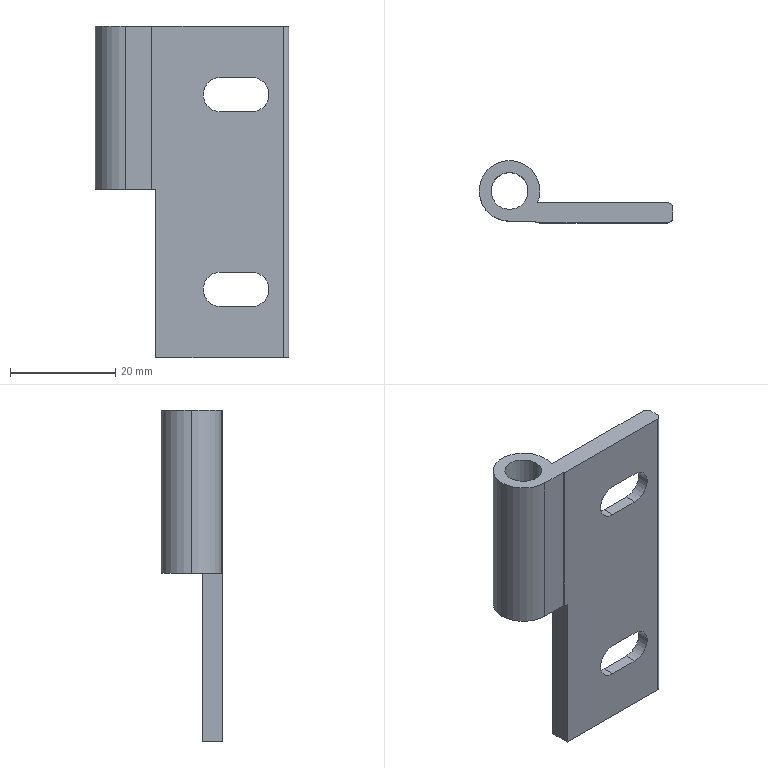Part | NX | features BREP 1 | 1 solid | 38 faces | box 36.75 x 11.75 x 63 mm | volume 7446 mm3 | cylinder 19 | plane 19 | commonest cylinder face diameters 6.5 x6 11 x6 11.5 x3 2 x2 7 x2
STEP:
#1=CARTESIAN_POINT('',(12.5,-3.7,18.5));
#2=VERTEX_POINT('',#1);
#3=CARTESIAN_POINT('',(18.,-3.7,24.));
#4=VERTEX_POINT('',#3);
#5=CARTESIAN_POINT('',(18.,-3.7,18.5));
#6=DIRECTION('',(0.,1.,0.));
#7=DIRECTION('',(-1.,0.,0.));
#8=AXIS2_PLACEMENT_3D('',#5,#6,#7);
#9=CIRCLE('',#8,5.5);
#10=EDGE_CURVE('',#2,#4,#9,.T.);
#11=ORIENTED_EDGE('',*,*,#10,.F.);
#12=CARTESIAN_POINT('',(12.5,-2.2,18.5));
#13=VERTEX_POINT('',#12);
#14=CARTESIAN_POINT('',(12.5,-3.7,18.5));
#15=DIRECTION('',(0.,1.,0.));
#16=VECTOR('',#15,1000.);
#17=LINE('',#14,#16);
#18=EDGE_CURVE('',#2,#13,#17,.T.);
#19=ORIENTED_EDGE('',*,*,#18,.T.);
#20=CARTESIAN_POINT('',(18.,-2.2,24.));
#21=VERTEX_POINT('',#20);
#22=CARTESIAN_POINT('',(18.,-2.2,18.5));
#23=DIRECTION('',(0.,1.,0.));
#24=DIRECTION('',(-1.,0.,0.));
#25=AXIS2_PLACEMENT_3D('',#22,#23,#24);
#26=CIRCLE('',#25,5.5);
#27=EDGE_CURVE('',#13,#21,#26,.T.);
#28=ORIENTED_EDGE('',*,*,#27,.T.);
#29=CARTESIAN_POINT('',(18.,-3.7,24.));
#30=DIRECTION('',(0.,1.,0.));
#31=VECTOR('',#30,1000.);
#32=LINE('',#29,#31);
#33=EDGE_CURVE('',#4,#21,#32,.T.);
#34=ORIENTED_EDGE('',*,*,#33,.F.);
#35=EDGE_LOOP('',(#11,#19,#28,#34));
#36=FACE_BOUND('',#35,.T.);
#37=CARTESIAN_POINT('',(18.,-3.7,18.5));
#38=DIRECTION('',(0.,1.,0.));
#39=DIRECTION('',(-1.,0.,0.));
#40=AXIS2_PLACEMENT_3D('',#37,#38,#39);
#41=CYLINDRICAL_SURFACE('',#40,5.5);
#42=ADVANCED_FACE('',(#36),#41,.F.);
#43=CARTESIAN_POINT('',(12.5,-3.7,-18.5));
#44=VERTEX_POINT('',#43);
#45=CARTESIAN_POINT('',(18.,-3.7,-13.));
#46=VERTEX_POINT('',#45);
#47=CARTESIAN_POINT('',(18.,-3.7,-18.5));
#48=DIRECTION('',(0.,1.,0.));
#49=DIRECTION('',(-1.,0.,0.));
#50=AXIS2_PLACEMENT_3D('',#47,#48,#49);
#51=CIRCLE('',#50,5.5);
#52=EDGE_CURVE('',#44,#46,#51,.T.);
#53=ORIENTED_EDGE('',*,*,#52,.F.);
#54=CARTESIAN_POINT('',(12.5,-2.2,-18.5));
#55=VERTEX_POINT('',#54);
#56=CARTESIAN_POINT('',(12.5,-3.7,-18.5));
#57=DIRECTION('',(0.,1.,0.));
#58=VECTOR('',#57,1000.);
#59=LINE('',#56,#58);
#60=EDGE_CURVE('',#44,#55,#59,.T.);
#61=ORIENTED_EDGE('',*,*,#60,.T.);
#62=CARTESIAN_POINT('',(18.,-2.2,-13.));
#63=VERTEX_POINT('',#62);
#64=CARTESIAN_POINT('',(18.,-2.2,-18.5));
#65=DIRECTION('',(0.,1.,0.));
#66=DIRECTION('',(-1.,0.,0.));
#67=AXIS2_PLACEMENT_3D('',#64,#65,#66);
#68=CIRCLE('',#67,5.5);
#69=EDGE_CURVE('',#55,#63,#68,.T.);
#70=ORIENTED_EDGE('',*,*,#69,.T.);
#71=CARTESIAN_POINT('',(18.,-3.7,-13.));
#72=DIRECTION('',(0.,1.,0.));
#73=VECTOR('',#72,1000.);
#74=LINE('',#71,#73);
#75=EDGE_CURVE('',#46,#63,#74,.T.);
#76=ORIENTED_EDGE('',*,*,#75,.F.);
#77=EDGE_LOOP('',(#53,#61,#70,#76));
#78=FACE_BOUND('',#77,.T.);
#79=CARTESIAN_POINT('',(18.,-3.7,-18.5));
#80=DIRECTION('',(0.,1.,0.));
#81=DIRECTION('',(-1.,0.,0.));
#82=AXIS2_PLACEMENT_3D('',#79,#80,#81);
#83=CYLINDRICAL_SURFACE('',#82,5.5);
#84=ADVANCED_FACE('',(#78),#83,.F.);
#85=CARTESIAN_POINT('',(-3.5,0.,31.5));
#86=VERTEX_POINT('',#85);
#87=CARTESIAN_POINT('',(3.5,0.,31.5));
#88=VERTEX_POINT('',#87);
#89=CARTESIAN_POINT('',(0.,0.,31.5));
#90=DIRECTION('',(0.,0.,1.));
#91=DIRECTION('',(1.,0.,0.));
#92=AXIS2_PLACEMENT_3D('',#89,#90,#91);
#93=CIRCLE('',#92,3.5);
#94=EDGE_CURVE('',#86,#88,#93,.T.);
#95=ORIENTED_EDGE('',*,*,#94,.T.);
#96=CARTESIAN_POINT('',(3.5,0.,0.5));
#97=VERTEX_POINT('',#96);
#98=CARTESIAN_POINT('',(3.5,0.,31.5));
#99=DIRECTION('',(0.,0.,-1.));
#100=VECTOR('',#99,1000.);
#101=LINE('',#98,#100);
#102=EDGE_CURVE('',#88,#97,#101,.T.);
#103=ORIENTED_EDGE('',*,*,#102,.T.);
#104=CARTESIAN_POINT('',(-3.5,0.,0.5));
#105=VERTEX_POINT('',#104);
#106=CARTESIAN_POINT('',(0.,0.,0.5));
#107=DIRECTION('',(0.,0.,1.));
#108=DIRECTION('',(1.,0.,0.));
#109=AXIS2_PLACEMENT_3D('',#106,#107,#108);
#110=CIRCLE('',#109,3.5);
#111=EDGE_CURVE('',#105,#97,#110,.T.);
#112=ORIENTED_EDGE('',*,*,#111,.F.);
#113=CARTESIAN_POINT('',(-3.5,0.,31.5));
#114=DIRECTION('',(0.,0.,-1.));
#115=VECTOR('',#114,1000.);
#116=LINE('',#113,#115);
#117=EDGE_CURVE('',#86,#105,#116,.T.);
#118=ORIENTED_EDGE('',*,*,#117,.F.);
#119=EDGE_LOOP('',(#95,#103,#112,#118));
#120=FACE_BOUND('',#119,.T.);
#121=CARTESIAN_POINT('',(0.,0.,31.5));
#122=DIRECTION('',(0.,0.,-1.));
#123=DIRECTION('',(-1.,0.,0.));
#124=AXIS2_PLACEMENT_3D('',#121,#122,#123);
#125=CYLINDRICAL_SURFACE('',#124,3.5);
#126=ADVANCED_FACE('',(#120),#125,.F.);
#127=CARTESIAN_POINT('',(5.75,0.,31.5));
#128=VERTEX_POINT('',#127);
#129=CARTESIAN_POINT('',(-5.75,0.,31.5));
#130=VERTEX_POINT('',#129);
#131=CARTESIAN_POINT('',(0.,0.,31.5));
#132=DIRECTION('',(0.,0.,1.));
#133=DIRECTION('',(1.,0.,0.));
#134=AXIS2_PLACEMENT_3D('',#131,#132,#133);
#135=CIRCLE('',#134,5.75);
#136=EDGE_CURVE('',#128,#130,#135,.T.);
#137=ORIENTED_EDGE('',*,*,#136,.F.);
#138=CARTESIAN_POINT('',(5.75,0.,0.5));
#139=VERTEX_POINT('',#138);
#140=CARTESIAN_POINT('',(5.75,0.,31.5));
#141=DIRECTION('',(0.,0.,-1.));
#142=VECTOR('',#141,1000.);
#143=LINE('',#140,#142);
#144=EDGE_CURVE('',#128,#139,#143,.T.);
#145=ORIENTED_EDGE('',*,*,#144,.T.);
#146=CARTESIAN_POINT('',(-5.75,0.,0.5));
#147=VERTEX_POINT('',#146);
#148=CARTESIAN_POINT('',(0.,0.,0.5));
#149=DIRECTION('',(0.,0.,1.));
#150=DIRECTION('',(1.,0.,0.));
#151=AXIS2_PLACEMENT_3D('',#148,#149,#150);
#152=CIRCLE('',#151,5.75);
#153=EDGE_CURVE('',#139,#147,#152,.T.);
#154=ORIENTED_EDGE('',*,*,#153,.T.);
#155=CARTESIAN_POINT('',(-5.75,0.,31.5));
#156=DIRECTION('',(0.,0.,-1.));
#157=VECTOR('',#156,1000.);
#158=LINE('',#155,#157);
#159=EDGE_CURVE('',#130,#147,#158,.T.);
#160=ORIENTED_EDGE('',*,*,#159,.F.);
#161=EDGE_LOOP('',(#137,#145,#154,#160));
#162=FACE_BOUND('',#161,.T.);
#163=CARTESIAN_POINT('',(0.,0.,31.5));
#164=DIRECTION('',(0.,0.,-1.));
#165=DIRECTION('',(-1.,0.,0.));
#166=AXIS2_PLACEMENT_3D('',#163,#164,#165);
#167=CYLINDRICAL_SURFACE('',#166,5.75);
#168=ADVANCED_FACE('',(#162),#167,.T.);
#169=CARTESIAN_POINT('',(0.,-5.75,31.5));
#170=VERTEX_POINT('',#169);
#171=CARTESIAN_POINT('',(0.,0.,31.5));
#172=DIRECTION('',(0.,0.,1.));
#173=DIRECTION('',(1.,0.,0.));
#174=AXIS2_PLACEMENT_3D('',#171,#172,#173);
#175=CIRCLE('',#174,5.75);
#176=EDGE_CURVE('',#130,#170,#175,.T.);
#177=ORIENTED_EDGE('',*,*,#176,.F.);
#178=ORIENTED_EDGE('',*,*,#159,.T.);
#179=CARTESIAN_POINT('',(0.,-5.75,0.5));
#180=VERTEX_POINT('',#179);
#181=CARTESIAN_POINT('',(0.,0.,0.5));
#182=DIRECTION('',(0.,0.,1.));
#183=DIRECTION('',(1.,0.,0.));
#184=AXIS2_PLACEMENT_3D('',#181,#182,#183);
#185=CIRCLE('',#184,5.75);
#186=EDGE_CURVE('',#147,#180,#185,.T.);
#187=ORIENTED_EDGE('',*,*,#186,.T.);
#188=CARTESIAN_POINT('',(0.,-5.75,31.5));
#189=DIRECTION('',(0.,0.,-1.));
#190=VECTOR('',#189,1000.);
#191=LINE('',#188,#190);
#192=EDGE_CURVE('',#170,#180,#191,.T.);
#193=ORIENTED_EDGE('',*,*,#192,.F.);
#194=EDGE_LOOP('',(#177,#178,#187,#193));
#195=FACE_BOUND('',#194,.T.);
#196=CARTESIAN_POINT('',(0.,0.,31.5));
#197=DIRECTION('',(0.,0.,-1.));
#198=DIRECTION('',(-1.,0.,0.));
#199=AXIS2_PLACEMENT_3D('',#196,#197,#198);
#200=CYLINDRICAL_SURFACE('',#199,5.75);
#201=ADVANCED_FACE('',(#195),#200,.T.);
#202=CARTESIAN_POINT('',(14.75,-6.,-18.5));
#203=VERTEX_POINT('',#202);
#204=CARTESIAN_POINT('',(18.,-6.,-15.25));
#205=VERTEX_POINT('',#204);
#206=CARTESIAN_POINT('',(18.,-6.,-18.5));
#207=DIRECTION('',(0.,1.,0.));
#208=DIRECTION('',(-1.,0.,0.));
#209=AXIS2_PLACEMENT_3D('',#206,#207,#208);
#210=CIRCLE('',#209,3.25);
#211=EDGE_CURVE('',#203,#205,#210,.T.);
#212=ORIENTED_EDGE('',*,*,#211,.F.);
#213=CARTESIAN_POINT('',(14.75,-3.7,-18.5));
#214=VERTEX_POINT('',#213);
#215=CARTESIAN_POINT('',(14.75,-6.,-18.5));
#216=DIRECTION('',(0.,1.,0.));
#217=VECTOR('',#216,1000.);
#218=LINE('',#215,#217);
#219=EDGE_CURVE('',#203,#214,#218,.T.);
#220=ORIENTED_EDGE('',*,*,#219,.T.);
#221=CARTESIAN_POINT('',(18.,-3.7,-15.25));
#222=VERTEX_POINT('',#221);
#223=CARTESIAN_POINT('',(18.,-3.7,-18.5));
#224=DIRECTION('',(0.,-1.,0.));
#225=DIRECTION('',(-1.,0.,0.));
#226=AXIS2_PLACEMENT_3D('',#223,#224,#225);
#227=CIRCLE('',#226,3.25);
#228=EDGE_CURVE('',#222,#214,#227,.T.);
#229=ORIENTED_EDGE('',*,*,#228,.F.);
#230=CARTESIAN_POINT('',(18.,-6.,-15.25));
#231=DIRECTION('',(0.,1.,0.));
#232=VECTOR('',#231,1000.);
#233=LINE('',#230,#232);
#234=EDGE_CURVE('',#205,#222,#233,.T.);
#235=ORIENTED_EDGE('',*,*,#234,.F.);
#236=EDGE_LOOP('',(#212,#220,#229,#235));
#237=FACE_BOUND('',#236,.T.);
#238=CARTESIAN_POINT('',(18.,-6.,-18.5));
#239=DIRECTION('',(0.,1.,0.));
#240=DIRECTION('',(-1.,0.,0.));
#241=AXIS2_PLACEMENT_3D('',#238,#239,#240);
#242=CYLINDRICAL_SURFACE('',#241,3.25);
#243=ADVANCED_FACE('',(#237),#242,.F.);
#244=CARTESIAN_POINT('',(14.75,-6.,18.5));
#245=VERTEX_POINT('',#244);
#246=CARTESIAN_POINT('',(18.,-6.,21.75));
#247=VERTEX_POINT('',#246);
#248=CARTESIAN_POINT('',(18.,-6.,18.5));
#249=DIRECTION('',(0.,1.,0.));
#250=DIRECTION('',(-1.,0.,0.));
#251=AXIS2_PLACEMENT_3D('',#248,#249,#250);
#252=CIRCLE('',#251,3.25);
#253=EDGE_CURVE('',#245,#247,#252,.T.);
#254=ORIENTED_EDGE('',*,*,#253,.F.);
#255=CARTESIAN_POINT('',(14.75,-3.7,18.5));
#256=VERTEX_POINT('',#255);
#257=CARTESIAN_POINT('',(14.75,-6.,18.5));
#258=DIRECTION('',(0.,1.,0.));
#259=VECTOR('',#258,1000.);
#260=LINE('',#257,#259);
#261=EDGE_CURVE('',#245,#256,#260,.T.);
#262=ORIENTED_EDGE('',*,*,#261,.T.);
#263=CARTESIAN_POINT('',(18.,-3.7,21.75));
#264=VERTEX_POINT('',#263);
#265=CARTESIAN_POINT('',(18.,-3.7,18.5));
#266=DIRECTION('',(0.,-1.,0.));
#267=DIRECTION('',(-1.,0.,0.));
#268=AXIS2_PLACEMENT_3D('',#265,#266,#267);
#269=CIRCLE('',#268,3.25);
#270=EDGE_CURVE('',#264,#256,#269,.T.);
#271=ORIENTED_EDGE('',*,*,#270,.F.);
#272=CARTESIAN_POINT('',(18.,-6.,21.75));
#273=DIRECTION('',(0.,1.,0.));
#274=VECTOR('',#273,1000.);
#275=LINE('',#272,#274);
#276=EDGE_CURVE('',#247,#264,#275,.T.);
#277=ORIENTED_EDGE('',*,*,#276,.F.);
#278=EDGE_LOOP('',(#254,#262,#271,#277));
#279=FACE_BOUND('',#278,.T.);
#280=CARTESIAN_POINT('',(18.,-6.,18.5));
#281=DIRECTION('',(0.,1.,0.));
#282=DIRECTION('',(-1.,0.,0.));
#283=AXIS2_PLACEMENT_3D('',#280,#281,#282);
#284=CYLINDRICAL_SURFACE('',#283,3.25);
#285=ADVANCED_FACE('',(#279),#284,.F.);
#286=ORIENTED_EDGE('',*,*,#261,.F.);
#287=CARTESIAN_POINT('',(18.,-6.,15.25));
#288=VERTEX_POINT('',#287);
#289=CARTESIAN_POINT('',(18.,-6.,18.5));
#290=DIRECTION('',(0.,1.,0.));
#291=DIRECTION('',(-1.,0.,0.));
#292=AXIS2_PLACEMENT_3D('',#289,#290,#291);
#293=CIRCLE('',#292,3.25);
#294=EDGE_CURVE('',#288,#245,#293,.T.);
#295=ORIENTED_EDGE('',*,*,#294,.F.);
#296=CARTESIAN_POINT('',(18.,-3.7,15.25));
#297=VERTEX_POINT('',#296);
#298=CARTESIAN_POINT('',(18.,-6.,15.25));
#299=DIRECTION('',(0.,1.,0.));
#300=VECTOR('',#299,1000.);
#301=LINE('',#298,#300);
#302=EDGE_CURVE('',#288,#297,#301,.T.);
#303=ORIENTED_EDGE('',*,*,#302,.T.);
#304=CARTESIAN_POINT('',(18.,-3.7,18.5));
#305=DIRECTION('',(0.,-1.,0.));
#306=DIRECTION('',(-1.,0.,0.));
#307=AXIS2_PLACEMENT_3D('',#304,#305,#306);
#308=CIRCLE('',#307,3.25);
#309=EDGE_CURVE('',#256,#297,#308,.T.);
#310=ORIENTED_EDGE('',*,*,#309,.F.);
#311=EDGE_LOOP('',(#286,#295,#303,#310));
#312=FACE_BOUND('',#311,.T.);
#313=CARTESIAN_POINT('',(18.,-6.,18.5));
#314=DIRECTION('',(0.,1.,0.));
#315=DIRECTION('',(-1.,0.,0.));
#316=AXIS2_PLACEMENT_3D('',#313,#314,#315);
#317=CYLINDRICAL_SURFACE('',#316,3.25);
#318=ADVANCED_FACE('',(#312),#317,.F.);
#319=CARTESIAN_POINT('',(24.,-3.7,15.25));
#320=VERTEX_POINT('',#319);
#321=CARTESIAN_POINT('',(18.,-3.7,15.25));
#322=DIRECTION('',(1.,0.,0.));
#323=VECTOR('',#322,1000.);
#324=LINE('',#321,#323);
#325=EDGE_CURVE('',#297,#320,#324,.T.);
#326=ORIENTED_EDGE('',*,*,#325,.F.);
#327=ORIENTED_EDGE('',*,*,#302,.F.);
#328=CARTESIAN_POINT('',(24.,-6.,15.25));
#329=VERTEX_POINT('',#328);
#330=CARTESIAN_POINT('',(18.,-6.,15.25));
#331=DIRECTION('',(-1.,0.,0.));
#332=VECTOR('',#331,1000.);
#333=LINE('',#330,#332);
#334=EDGE_CURVE('',#329,#288,#333,.T.);
#335=ORIENTED_EDGE('',*,*,#334,.F.);
#336=CARTESIAN_POINT('',(24.,-6.,15.25));
#337=DIRECTION('',(0.,1.,0.));
#338=VECTOR('',#337,1000.);
#339=LINE('',#336,#338);
#340=EDGE_CURVE('',#329,#320,#339,.T.);
#341=ORIENTED_EDGE('',*,*,#340,.T.);
#342=EDGE_LOOP('',(#326,#327,#335,#341));
#343=FACE_BOUND('',#342,.T.);
#344=CARTESIAN_POINT('',(18.,-6.,15.25));
#345=DIRECTION('',(0.,0.,-1.));
#346=DIRECTION('',(0.,-1.,0.));
#347=AXIS2_PLACEMENT_3D('',#344,#345,#346);
#348=PLANE('',#347);
#349=ADVANCED_FACE('',(#343),#348,.F.);
#350=CARTESIAN_POINT('',(24.,-3.7,21.75));
#351=VERTEX_POINT('',#350);
#352=CARTESIAN_POINT('',(24.,-3.7,18.5));
#353=DIRECTION('',(0.,-1.,0.));
#354=DIRECTION('',(-1.,0.,0.));
#355=AXIS2_PLACEMENT_3D('',#352,#353,#354);
#356=CIRCLE('',#355,3.25);
#357=EDGE_CURVE('',#320,#351,#356,.T.);
#358=ORIENTED_EDGE('',*,*,#357,.F.);
#359=ORIENTED_EDGE('',*,*,#340,.F.);
#360=CARTESIAN_POINT('',(24.,-6.,21.75));
#361=VERTEX_POINT('',#360);
#362=CARTESIAN_POINT('',(24.,-6.,18.5));
#363=DIRECTION('',(0.,1.,0.));
#364=DIRECTION('',(-1.,0.,0.));
#365=AXIS2_PLACEMENT_3D('',#362,#363,#364);
#366=CIRCLE('',#365,3.25);
#367=EDGE_CURVE('',#361,#329,#366,.T.);
#368=ORIENTED_EDGE('',*,*,#367,.F.);
#369=CARTESIAN_POINT('',(24.,-6.,21.75));
#370=DIRECTION('',(0.,1.,0.));
#371=VECTOR('',#370,1000.);
#372=LINE('',#369,#371);
#373=EDGE_CURVE('',#361,#351,#372,.T.);
#374=ORIENTED_EDGE('',*,*,#373,.T.);
#375=EDGE_LOOP('',(#358,#359,#368,#374));
#376=FACE_BOUND('',#375,.T.);
#377=CARTESIAN_POINT('',(24.,-6.,18.5));
#378=DIRECTION('',(0.,1.,0.));
#379=DIRECTION('',(-1.,0.,0.));
#380=AXIS2_PLACEMENT_3D('',#377,#378,#379);
#381=CYLINDRICAL_SURFACE('',#380,3.25);
#382=ADVANCED_FACE('',(#376),#381,.F.);
#383=CARTESIAN_POINT('',(18.,-3.7,21.75));
#384=DIRECTION('',(-1.,0.,0.));
#385=VECTOR('',#384,1000.);
#386=LINE('',#383,#385);
#387=EDGE_CURVE('',#351,#264,#386,.T.);
#388=ORIENTED_EDGE('',*,*,#387,.F.);
#389=ORIENTED_EDGE('',*,*,#373,.F.);
#390=CARTESIAN_POINT('',(18.,-6.,21.75));
#391=DIRECTION('',(1.,0.,0.));
#392=VECTOR('',#391,1000.);
#393=LINE('',#390,#392);
#394=EDGE_CURVE('',#247,#361,#393,.T.);
#395=ORIENTED_EDGE('',*,*,#394,.F.);
#396=ORIENTED_EDGE('',*,*,#276,.T.);
#397=EDGE_LOOP('',(#388,#389,#395,#396));
#398=FACE_BOUND('',#397,.T.);
#399=CARTESIAN_POINT('',(18.,-6.,21.75));
#400=DIRECTION('',(0.,0.,1.));
#401=DIRECTION('',(1.,0.,0.));
#402=AXIS2_PLACEMENT_3D('',#399,#400,#401);
#403=PLANE('',#402);
#404=ADVANCED_FACE('',(#398),#403,.F.);
#405=ORIENTED_EDGE('',*,*,#219,.F.);
#406=CARTESIAN_POINT('',(18.,-6.,-21.75));
#407=VERTEX_POINT('',#406);
#408=CARTESIAN_POINT('',(18.,-6.,-18.5));
#409=DIRECTION('',(0.,1.,0.));
#410=DIRECTION('',(-1.,0.,0.));
#411=AXIS2_PLACEMENT_3D('',#408,#409,#410);
#412=CIRCLE('',#411,3.25);
#413=EDGE_CURVE('',#407,#203,#412,.T.);
#414=ORIENTED_EDGE('',*,*,#413,.F.);
#415=CARTESIAN_POINT('',(18.,-3.7,-21.75));
#416=VERTEX_POINT('',#415);
#417=CARTESIAN_POINT('',(18.,-6.,-21.75));
#418=DIRECTION('',(0.,1.,0.));
#419=VECTOR('',#418,1000.);
#420=LINE('',#417,#419);
#421=EDGE_CURVE('',#407,#416,#420,.T.);
#422=ORIENTED_EDGE('',*,*,#421,.T.);
#423=CARTESIAN_POINT('',(18.,-3.7,-18.5));
#424=DIRECTION('',(0.,-1.,0.));
#425=DIRECTION('',(-1.,0.,0.));
#426=AXIS2_PLACEMENT_3D('',#423,#424,#425);
#427=CIRCLE('',#426,3.25);
#428=EDGE_CURVE('',#214,#416,#427,.T.);
#429=ORIENTED_EDGE('',*,*,#428,.F.);
#430=EDGE_LOOP('',(#405,#414,#422,#429));
#431=FACE_BOUND('',#430,.T.);
#432=CARTESIAN_POINT('',(18.,-6.,-18.5));
#433=DIRECTION('',(0.,1.,0.));
#434=DIRECTION('',(-1.,0.,0.));
#435=AXIS2_PLACEMENT_3D('',#432,#433,#434);
#436=CYLINDRICAL_SURFACE('',#435,3.25);
#437=ADVANCED_FACE('',(#431),#436,.F.);
#438=CARTESIAN_POINT('',(24.,-3.7,-21.75));
#439=VERTEX_POINT('',#438);
#440=CARTESIAN_POINT('',(18.,-3.7,-21.75));
#441=DIRECTION('',(1.,0.,0.));
#442=VECTOR('',#441,1000.);
#443=LINE('',#440,#442);
#444=EDGE_CURVE('',#416,#439,#443,.T.);
#445=ORIENTED_EDGE('',*,*,#444,.F.);
#446=ORIENTED_EDGE('',*,*,#421,.F.);
#447=CARTESIAN_POINT('',(24.,-6.,-21.75));
#448=VERTEX_POINT('',#447);
#449=CARTESIAN_POINT('',(18.,-6.,-21.75));
#450=DIRECTION('',(-1.,0.,0.));
#451=VECTOR('',#450,1000.);
#452=LINE('',#449,#451);
#453=EDGE_CURVE('',#448,#407,#452,.T.);
#454=ORIENTED_EDGE('',*,*,#453,.F.);
#455=CARTESIAN_POINT('',(24.,-6.,-21.75));
#456=DIRECTION('',(0.,1.,0.));
#457=VECTOR('',#456,1000.);
#458=LINE('',#455,#457);
#459=EDGE_CURVE('',#448,#439,#458,.T.);
#460=ORIENTED_EDGE('',*,*,#459,.T.);
#461=EDGE_LOOP('',(#445,#446,#454,#460));
#462=FACE_BOUND('',#461,.T.);
#463=CARTESIAN_POINT('',(18.,-6.,-21.75));
#464=DIRECTION('',(0.,0.,-1.));
#465=DIRECTION('',(0.,-1.,0.));
#466=AXIS2_PLACEMENT_3D('',#463,#464,#465);
#467=PLANE('',#466);
#468=ADVANCED_FACE('',(#462),#467,.F.);
#469=CARTESIAN_POINT('',(24.,-3.7,-15.25));
#470=VERTEX_POINT('',#469);
#471=CARTESIAN_POINT('',(24.,-3.7,-18.5));
#472=DIRECTION('',(0.,-1.,0.));
#473=DIRECTION('',(-1.,0.,0.));
#474=AXIS2_PLACEMENT_3D('',#471,#472,#473);
#475=CIRCLE('',#474,3.25);
#476=EDGE_CURVE('',#439,#470,#475,.T.);
#477=ORIENTED_EDGE('',*,*,#476,.F.);
#478=ORIENTED_EDGE('',*,*,#459,.F.);
#479=CARTESIAN_POINT('',(24.,-6.,-15.25));
#480=VERTEX_POINT('',#479);
#481=CARTESIAN_POINT('',(24.,-6.,-18.5));
#482=DIRECTION('',(0.,1.,0.));
#483=DIRECTION('',(-1.,0.,0.));
#484=AXIS2_PLACEMENT_3D('',#481,#482,#483);
#485=CIRCLE('',#484,3.25);
#486=EDGE_CURVE('',#480,#448,#485,.T.);
#487=ORIENTED_EDGE('',*,*,#486,.F.);
#488=CARTESIAN_POINT('',(24.,-6.,-15.25));
#489=DIRECTION('',(0.,1.,0.));
#490=VECTOR('',#489,1000.);
#491=LINE('',#488,#490);
#492=EDGE_CURVE('',#480,#470,#491,.T.);
#493=ORIENTED_EDGE('',*,*,#492,.T.);
#494=EDGE_LOOP('',(#477,#478,#487,#493));
#495=FACE_BOUND('',#494,.T.);
#496=CARTESIAN_POINT('',(24.,-6.,-18.5));
#497=DIRECTION('',(0.,1.,0.));
#498=DIRECTION('',(-1.,0.,0.));
#499=AXIS2_PLACEMENT_3D('',#496,#497,#498);
#500=CYLINDRICAL_SURFACE('',#499,3.25);
#501=ADVANCED_FACE('',(#495),#500,.F.);
#502=CARTESIAN_POINT('',(18.,-3.7,-15.25));
#503=DIRECTION('',(-1.,0.,0.));
#504=VECTOR('',#503,1000.);
#505=LINE('',#502,#504);
#506=EDGE_CURVE('',#470,#222,#505,.T.);
#507=ORIENTED_EDGE('',*,*,#506,.F.);
#508=ORIENTED_EDGE('',*,*,#492,.F.);
#509=CARTESIAN_POINT('',(18.,-6.,-15.25));
#510=DIRECTION('',(1.,0.,0.));
#511=VECTOR('',#510,1000.);
#512=LINE('',#509,#511);
#513=EDGE_CURVE('',#205,#480,#512,.T.);
#514=ORIENTED_EDGE('',*,*,#513,.F.);
#515=ORIENTED_EDGE('',*,*,#234,.T.);
#516=EDGE_LOOP('',(#507,#508,#514,#515));
#517=FACE_BOUND('',#516,.T.);
#518=CARTESIAN_POINT('',(18.,-6.,-15.25));
#519=DIRECTION('',(0.,0.,1.));
#520=DIRECTION('',(1.,0.,0.));
#521=AXIS2_PLACEMENT_3D('',#518,#519,#520);
#522=PLANE('',#521);
#523=ADVANCED_FACE('',(#517),#522,.F.);
#524=CARTESIAN_POINT('',(5.,-6.,31.5));
#525=VERTEX_POINT('',#524);
#526=CARTESIAN_POINT('',(30.,-6.,31.5));
#527=VERTEX_POINT('',#526);
#528=CARTESIAN_POINT('',(5.,-6.,31.5));
#529=DIRECTION('',(1.,0.,0.));
#530=VECTOR('',#529,1000.);
#531=LINE('',#528,#530);
#532=EDGE_CURVE('',#525,#527,#531,.T.);
#533=ORIENTED_EDGE('',*,*,#532,.T.);
#534=CARTESIAN_POINT('',(31.,-5.,31.5));
#535=VERTEX_POINT('',#534);
#536=CARTESIAN_POINT('',(30.,-5.,31.5));
#537=DIRECTION('',(0.,0.,1.));
#538=DIRECTION('',(1.,0.,0.));
#539=AXIS2_PLACEMENT_3D('',#536,#537,#538);
#540=CIRCLE('',#539,1.);
#541=EDGE_CURVE('',#527,#535,#540,.T.);
#542=ORIENTED_EDGE('',*,*,#541,.T.);
#543=CARTESIAN_POINT('',(31.,-3.2,31.5));
#544=VERTEX_POINT('',#543);
#545=CARTESIAN_POINT('',(31.,-6.,31.5));
#546=DIRECTION('',(0.,1.,0.));
#547=VECTOR('',#546,1000.);
#548=LINE('',#545,#547);
#549=EDGE_CURVE('',#535,#544,#548,.T.);
#550=ORIENTED_EDGE('',*,*,#549,.T.);
#551=CARTESIAN_POINT('',(30.,-2.2,31.5));
#552=VERTEX_POINT('',#551);
#553=CARTESIAN_POINT('',(30.,-3.2,31.5));
#554=DIRECTION('',(0.,0.,1.));
#555=DIRECTION('',(1.,0.,0.));
#556=AXIS2_PLACEMENT_3D('',#553,#554,#555);
#557=CIRCLE('',#556,1.);
#558=EDGE_CURVE('',#544,#552,#557,.T.);
#559=ORIENTED_EDGE('',*,*,#558,.T.);
#560=CARTESIAN_POINT('',(5.312,-2.2,31.5));
#561=VERTEX_POINT('',#560);
#562=CARTESIAN_POINT('',(31.,-2.2,31.5));
#563=DIRECTION('',(-1.,0.,0.));
#564=VECTOR('',#563,1000.);
#565=LINE('',#562,#564);
#566=EDGE_CURVE('',#552,#561,#565,.T.);
#567=ORIENTED_EDGE('',*,*,#566,.T.);
#568=CARTESIAN_POINT('',(0.,0.,31.5));
#569=DIRECTION('',(0.,0.,1.));
#570=DIRECTION('',(1.,0.,0.));
#571=AXIS2_PLACEMENT_3D('',#568,#569,#570);
#572=CIRCLE('',#571,5.75);
#573=EDGE_CURVE('',#561,#128,#572,.T.);
#574=ORIENTED_EDGE('',*,*,#573,.T.);
#575=ORIENTED_EDGE('',*,*,#136,.T.);
#576=ORIENTED_EDGE('',*,*,#176,.T.);
#577=CARTESIAN_POINT('',(5.,-5.75,31.5));
#578=VERTEX_POINT('',#577);
#579=CARTESIAN_POINT('',(0.,-5.75,31.5));
#580=DIRECTION('',(1.,0.,0.));
#581=VECTOR('',#580,1000.);
#582=LINE('',#579,#581);
#583=EDGE_CURVE('',#170,#578,#582,.T.);
#584=ORIENTED_EDGE('',*,*,#583,.T.);
#585=CARTESIAN_POINT('',(5.,-5.75,31.5));
#586=DIRECTION('',(0.,-1.,0.));
#587=VECTOR('',#586,1000.);
#588=LINE('',#585,#587);
#589=EDGE_CURVE('',#578,#525,#588,.T.);
#590=ORIENTED_EDGE('',*,*,#589,.T.);
#591=EDGE_LOOP('',(#533,#542,#550,#559,#567,#574,#575,#576,#584,#590));
#592=FACE_BOUND('',#591,.T.);
#593=ORIENTED_EDGE('',*,*,#94,.F.);
#594=CARTESIAN_POINT('',(0.,0.,31.5));
#595=DIRECTION('',(0.,0.,1.));
#596=DIRECTION('',(1.,0.,0.));
#597=AXIS2_PLACEMENT_3D('',#594,#595,#596);
#598=CIRCLE('',#597,3.5);
#599=EDGE_CURVE('',#88,#86,#598,.T.);
#600=ORIENTED_EDGE('',*,*,#599,.F.);
#601=EDGE_LOOP('',(#593,#600));
#602=FACE_BOUND('',#601,.T.);
#603=CARTESIAN_POINT('',(0.,0.,31.5));
#604=DIRECTION('',(0.,0.,1.));
#605=DIRECTION('',(1.,0.,0.));
#606=AXIS2_PLACEMENT_3D('',#603,#604,#605);
#607=PLANE('',#606);
#608=ADVANCED_FACE('',(#592,#602),#607,.T.);
#609=CARTESIAN_POINT('',(5.75,-6.,-31.5));
#610=VERTEX_POINT('',#609);
#611=CARTESIAN_POINT('',(30.,-6.,-31.5));
#612=VERTEX_POINT('',#611);
#613=CARTESIAN_POINT('',(5.,-6.,-31.5));
#614=DIRECTION('',(1.,0.,0.));
#615=VECTOR('',#614,1000.);
#616=LINE('',#613,#615);
#617=EDGE_CURVE('',#610,#612,#616,.T.);
#618=ORIENTED_EDGE('',*,*,#617,.F.);
#619=CARTESIAN_POINT('',(5.75,-2.2,-31.5));
#620=VERTEX_POINT('',#619);
#621=CARTESIAN_POINT('',(5.75,5.75,-31.5));
#622=DIRECTION('',(0.,-1.,0.));
#623=VECTOR('',#622,1000.);
#624=LINE('',#621,#623);
#625=EDGE_CURVE('',#620,#610,#624,.T.);
#626=ORIENTED_EDGE('',*,*,#625,.F.);
#627=CARTESIAN_POINT('',(30.,-2.2,-31.5));
#628=VERTEX_POINT('',#627);
#629=CARTESIAN_POINT('',(31.,-2.2,-31.5));
#630=DIRECTION('',(-1.,0.,0.));
#631=VECTOR('',#630,1000.);
#632=LINE('',#629,#631);
#633=EDGE_CURVE('',#628,#620,#632,.T.);
#634=ORIENTED_EDGE('',*,*,#633,.F.);
#635=CARTESIAN_POINT('',(31.,-3.2,-31.5));
#636=VERTEX_POINT('',#635);
#637=CARTESIAN_POINT('',(30.,-3.2,-31.5));
#638=DIRECTION('',(0.,0.,-1.));
#639=DIRECTION('',(1.,0.,0.));
#640=AXIS2_PLACEMENT_3D('',#637,#638,#639);
#641=CIRCLE('',#640,1.);
#642=EDGE_CURVE('',#628,#636,#641,.T.);
#643=ORIENTED_EDGE('',*,*,#642,.T.);
#644=CARTESIAN_POINT('',(31.,-5.,-31.5));
#645=VERTEX_POINT('',#644);
#646=CARTESIAN_POINT('',(31.,-6.,-31.5));
#647=DIRECTION('',(0.,1.,0.));
#648=VECTOR('',#647,1000.);
#649=LINE('',#646,#648);
#650=EDGE_CURVE('',#645,#636,#649,.T.);
#651=ORIENTED_EDGE('',*,*,#650,.F.);
#652=CARTESIAN_POINT('',(30.,-5.,-31.5));
#653=DIRECTION('',(0.,0.,-1.));
#654=DIRECTION('',(1.,0.,0.));
#655=AXIS2_PLACEMENT_3D('',#652,#653,#654);
#656=CIRCLE('',#655,1.);
#657=EDGE_CURVE('',#645,#612,#656,.T.);
#658=ORIENTED_EDGE('',*,*,#657,.T.);
#659=EDGE_LOOP('',(#618,#626,#634,#643,#651,#658));
#660=FACE_BOUND('',#659,.T.);
#661=CARTESIAN_POINT('',(0.,0.,-31.5));
#662=DIRECTION('',(0.,0.,1.));
#663=DIRECTION('',(1.,0.,0.));
#664=AXIS2_PLACEMENT_3D('',#661,#662,#663);
#665=PLANE('',#664);
#666=ADVANCED_FACE('',(#660),#665,.F.);
#667=ORIENTED_EDGE('',*,*,#144,.F.);
#668=ORIENTED_EDGE('',*,*,#573,.F.);
#669=CARTESIAN_POINT('',(5.312,-2.2,0.5));
#670=VERTEX_POINT('',#669);
#671=CARTESIAN_POINT('',(5.312,-2.2,31.5));
#672=DIRECTION('',(0.,0.,-1.));
#673=VECTOR('',#672,1000.);
#674=LINE('',#671,#673);
#675=EDGE_CURVE('',#561,#670,#674,.T.);
#676=ORIENTED_EDGE('',*,*,#675,.T.);
#677=CARTESIAN_POINT('',(0.,0.,0.5));
#678=DIRECTION('',(0.,0.,1.));
#679=DIRECTION('',(1.,0.,0.));
#680=AXIS2_PLACEMENT_3D('',#677,#678,#679);
#681=CIRCLE('',#680,5.75);
#682=EDGE_CURVE('',#670,#139,#681,.T.);
#683=ORIENTED_EDGE('',*,*,#682,.T.);
#684=EDGE_LOOP('',(#667,#668,#676,#683));
#685=FACE_BOUND('',#684,.T.);
#686=CARTESIAN_POINT('',(0.,0.,31.5));
#687=DIRECTION('',(0.,0.,-1.));
#688=DIRECTION('',(-1.,0.,0.));
#689=AXIS2_PLACEMENT_3D('',#686,#687,#688);
#690=CYLINDRICAL_SURFACE('',#689,5.75);
#691=ADVANCED_FACE('',(#685),#690,.T.);
#692=ORIENTED_EDGE('',*,*,#192,.T.);
#693=CARTESIAN_POINT('',(5.,-5.75,0.5));
#694=VERTEX_POINT('',#693);
#695=CARTESIAN_POINT('',(0.,-5.75,0.5));
#696=DIRECTION('',(1.,0.,0.));
#697=VECTOR('',#696,1000.);
#698=LINE('',#695,#697);
#699=EDGE_CURVE('',#180,#694,#698,.T.);
#700=ORIENTED_EDGE('',*,*,#699,.T.);
#701=CARTESIAN_POINT('',(5.,-5.75,31.5));
#702=DIRECTION('',(0.,0.,-1.));
#703=VECTOR('',#702,1000.);
#704=LINE('',#701,#703);
#705=EDGE_CURVE('',#578,#694,#704,.T.);
#706=ORIENTED_EDGE('',*,*,#705,.F.);
#707=ORIENTED_EDGE('',*,*,#583,.F.);
#708=EDGE_LOOP('',(#692,#700,#706,#707));
#709=FACE_BOUND('',#708,.T.);
#710=CARTESIAN_POINT('',(0.,-5.75,31.5));
#711=DIRECTION('',(0.,1.,0.));
#712=DIRECTION('',(1.,0.,0.));
#713=AXIS2_PLACEMENT_3D('',#710,#711,#712);
#714=PLANE('',#713);
#715=ADVANCED_FACE('',(#709),#714,.F.);
#716=ORIENTED_EDGE('',*,*,#705,.T.);
#717=CARTESIAN_POINT('',(5.,-6.,0.5));
#718=VERTEX_POINT('',#717);
#719=CARTESIAN_POINT('',(5.,-5.75,0.5));
#720=DIRECTION('',(0.,-1.,0.));
#721=VECTOR('',#720,1000.);
#722=LINE('',#719,#721);
#723=EDGE_CURVE('',#694,#718,#722,.T.);
#724=ORIENTED_EDGE('',*,*,#723,.T.);
#725=CARTESIAN_POINT('',(5.,-6.,31.5));
#726=DIRECTION('',(0.,0.,-1.));
#727=VECTOR('',#726,1000.);
#728=LINE('',#725,#727);
#729=EDGE_CURVE('',#525,#718,#728,.T.);
#730=ORIENTED_EDGE('',*,*,#729,.F.);
#731=ORIENTED_EDGE('',*,*,#589,.F.);
#732=EDGE_LOOP('',(#716,#724,#730,#731));
#733=FACE_BOUND('',#732,.T.);
#734=CARTESIAN_POINT('',(5.,-5.75,31.5));
#735=DIRECTION('',(1.,0.,0.));
#736=DIRECTION('',(0.,1.,0.));
#737=AXIS2_PLACEMENT_3D('',#734,#735,#736);
#738=PLANE('',#737);
#739=ADVANCED_FACE('',(#733),#738,.F.);
#740=ORIENTED_EDGE('',*,*,#729,.T.);
#741=CARTESIAN_POINT('',(5.75,-6.,0.5));
#742=VERTEX_POINT('',#741);
#743=CARTESIAN_POINT('',(-5.75,-6.,0.5));
#744=DIRECTION('',(-1.,0.,0.));
#745=VECTOR('',#744,1000.);
#746=LINE('',#743,#745);
#747=EDGE_CURVE('',#742,#718,#746,.T.);
#748=ORIENTED_EDGE('',*,*,#747,.F.);
#749=CARTESIAN_POINT('',(5.75,-6.,-31.5));
#750=DIRECTION('',(0.,0.,1.));
#751=VECTOR('',#750,1000.);
#752=LINE('',#749,#751);
#753=EDGE_CURVE('',#610,#742,#752,.T.);
#754=ORIENTED_EDGE('',*,*,#753,.F.);
#755=ORIENTED_EDGE('',*,*,#617,.T.);
#756=CARTESIAN_POINT('',(30.,-6.,31.5));
#757=DIRECTION('',(0.,0.,1.));
#758=VECTOR('',#757,1000.);
#759=LINE('',#756,#758);
#760=EDGE_CURVE('',#612,#527,#759,.T.);
#761=ORIENTED_EDGE('',*,*,#760,.T.);
#762=ORIENTED_EDGE('',*,*,#532,.F.);
#763=EDGE_LOOP('',(#740,#748,#754,#755,#761,#762));
#764=FACE_BOUND('',#763,.T.);
#765=ORIENTED_EDGE('',*,*,#334,.T.);
#766=ORIENTED_EDGE('',*,*,#294,.T.);
#767=ORIENTED_EDGE('',*,*,#253,.T.);
#768=ORIENTED_EDGE('',*,*,#394,.T.);
#769=ORIENTED_EDGE('',*,*,#367,.T.);
#770=EDGE_LOOP('',(#765,#766,#767,#768,#769));
#771=FACE_BOUND('',#770,.T.);
#772=ORIENTED_EDGE('',*,*,#453,.T.);
#773=ORIENTED_EDGE('',*,*,#413,.T.);
#774=ORIENTED_EDGE('',*,*,#211,.T.);
#775=ORIENTED_EDGE('',*,*,#513,.T.);
#776=ORIENTED_EDGE('',*,*,#486,.T.);
#777=EDGE_LOOP('',(#772,#773,#774,#775,#776));
#778=FACE_BOUND('',#777,.T.);
#779=CARTESIAN_POINT('',(5.,-6.,31.5));
#780=DIRECTION('',(0.,1.,0.));
#781=DIRECTION('',(1.,0.,0.));
#782=AXIS2_PLACEMENT_3D('',#779,#780,#781);
#783=PLANE('',#782);
#784=ADVANCED_FACE('',(#764,#771,#778),#783,.F.);
#785=ORIENTED_EDGE('',*,*,#549,.F.);
#786=CARTESIAN_POINT('',(31.,-5.,31.5));
#787=DIRECTION('',(0.,0.,-1.));
#788=VECTOR('',#787,1000.);
#789=LINE('',#786,#788);
#790=EDGE_CURVE('',#535,#645,#789,.T.);
#791=ORIENTED_EDGE('',*,*,#790,.T.);
#792=ORIENTED_EDGE('',*,*,#650,.T.);
#793=CARTESIAN_POINT('',(31.,-3.2,31.5));
#794=DIRECTION('',(0.,0.,1.));
#795=VECTOR('',#794,1000.);
#796=LINE('',#793,#795);
#797=EDGE_CURVE('',#636,#544,#796,.T.);
#798=ORIENTED_EDGE('',*,*,#797,.T.);
#799=EDGE_LOOP('',(#785,#791,#792,#798));
#800=FACE_BOUND('',#799,.T.);
#801=CARTESIAN_POINT('',(31.,-6.,31.5));
#802=DIRECTION('',(-1.,0.,0.));
#803=DIRECTION('',(0.,0.,1.));
#804=AXIS2_PLACEMENT_3D('',#801,#802,#803);
#805=PLANE('',#804);
#806=ADVANCED_FACE('',(#800),#805,.F.);
#807=CARTESIAN_POINT('',(5.75,-2.2,0.5));
#808=VERTEX_POINT('',#807);
#809=CARTESIAN_POINT('',(5.75,-2.2,31.5));
#810=DIRECTION('',(0.,0.,1.));
#811=VECTOR('',#810,1000.);
#812=LINE('',#809,#811);
#813=EDGE_CURVE('',#620,#808,#812,.T.);
#814=ORIENTED_EDGE('',*,*,#813,.T.);
#815=CARTESIAN_POINT('',(31.,-2.2,0.5));
#816=DIRECTION('',(-1.,0.,0.));
#817=VECTOR('',#816,1000.);
#818=LINE('',#815,#817);
#819=EDGE_CURVE('',#808,#670,#818,.T.);
#820=ORIENTED_EDGE('',*,*,#819,.T.);
#821=ORIENTED_EDGE('',*,*,#675,.F.);
#822=ORIENTED_EDGE('',*,*,#566,.F.);
#823=CARTESIAN_POINT('',(30.,-2.2,31.5));
#824=DIRECTION('',(0.,0.,-1.));
#825=VECTOR('',#824,1000.);
#826=LINE('',#823,#825);
#827=EDGE_CURVE('',#552,#628,#826,.T.);
#828=ORIENTED_EDGE('',*,*,#827,.T.);
#829=ORIENTED_EDGE('',*,*,#633,.T.);
#830=EDGE_LOOP('',(#814,#820,#821,#822,#828,#829));
#831=FACE_BOUND('',#830,.T.);
#832=CARTESIAN_POINT('',(24.,-2.2,24.));
#833=VERTEX_POINT('',#832);
#834=CARTESIAN_POINT('',(18.,-2.2,24.));
#835=DIRECTION('',(1.,0.,0.));
#836=VECTOR('',#835,1000.);
#837=LINE('',#834,#836);
#838=EDGE_CURVE('',#21,#833,#837,.T.);
#839=ORIENTED_EDGE('',*,*,#838,.F.);
#840=ORIENTED_EDGE('',*,*,#27,.F.);
#841=CARTESIAN_POINT('',(18.,-2.2,13.));
#842=VERTEX_POINT('',#841);
#843=CARTESIAN_POINT('',(18.,-2.2,18.5));
#844=DIRECTION('',(0.,1.,0.));
#845=DIRECTION('',(-1.,0.,0.));
#846=AXIS2_PLACEMENT_3D('',#843,#844,#845);
#847=CIRCLE('',#846,5.5);
#848=EDGE_CURVE('',#842,#13,#847,.T.);
#849=ORIENTED_EDGE('',*,*,#848,.F.);
#850=CARTESIAN_POINT('',(24.,-2.2,13.));
#851=VERTEX_POINT('',#850);
#852=CARTESIAN_POINT('',(18.,-2.2,13.));
#853=DIRECTION('',(-1.,0.,0.));
#854=VECTOR('',#853,1000.);
#855=LINE('',#852,#854);
#856=EDGE_CURVE('',#851,#842,#855,.T.);
#857=ORIENTED_EDGE('',*,*,#856,.F.);
#858=CARTESIAN_POINT('',(24.,-2.2,18.5));
#859=DIRECTION('',(0.,1.,0.));
#860=DIRECTION('',(-1.,0.,0.));
#861=AXIS2_PLACEMENT_3D('',#858,#859,#860);
#862=CIRCLE('',#861,5.5);
#863=EDGE_CURVE('',#833,#851,#862,.T.);
#864=ORIENTED_EDGE('',*,*,#863,.F.);
#865=EDGE_LOOP('',(#839,#840,#849,#857,#864));
#866=FACE_BOUND('',#865,.T.);
#867=CARTESIAN_POINT('',(24.,-2.2,-13.));
#868=VERTEX_POINT('',#867);
#869=CARTESIAN_POINT('',(18.,-2.2,-13.));
#870=DIRECTION('',(1.,0.,0.));
#871=VECTOR('',#870,1000.);
#872=LINE('',#869,#871);
#873=EDGE_CURVE('',#63,#868,#872,.T.);
#874=ORIENTED_EDGE('',*,*,#873,.F.);
#875=ORIENTED_EDGE('',*,*,#69,.F.);
#876=CARTESIAN_POINT('',(18.,-2.2,-24.));
#877=VERTEX_POINT('',#876);
#878=CARTESIAN_POINT('',(18.,-2.2,-18.5));
#879=DIRECTION('',(0.,1.,0.));
#880=DIRECTION('',(-1.,0.,0.));
#881=AXIS2_PLACEMENT_3D('',#878,#879,#880);
#882=CIRCLE('',#881,5.5);
#883=EDGE_CURVE('',#877,#55,#882,.T.);
#884=ORIENTED_EDGE('',*,*,#883,.F.);
#885=CARTESIAN_POINT('',(24.,-2.2,-24.));
#886=VERTEX_POINT('',#885);
#887=CARTESIAN_POINT('',(18.,-2.2,-24.));
#888=DIRECTION('',(-1.,0.,0.));
#889=VECTOR('',#888,1000.);
#890=LINE('',#887,#889);
#891=EDGE_CURVE('',#886,#877,#890,.T.);
#892=ORIENTED_EDGE('',*,*,#891,.F.);
#893=CARTESIAN_POINT('',(24.,-2.2,-18.5));
#894=DIRECTION('',(0.,1.,0.));
#895=DIRECTION('',(-1.,0.,0.));
#896=AXIS2_PLACEMENT_3D('',#893,#894,#895);
#897=CIRCLE('',#896,5.5);
#898=EDGE_CURVE('',#868,#886,#897,.T.);
#899=ORIENTED_EDGE('',*,*,#898,.F.);
#900=EDGE_LOOP('',(#874,#875,#884,#892,#899));
#901=FACE_BOUND('',#900,.T.);
#902=CARTESIAN_POINT('',(31.,-2.2,31.5));
#903=DIRECTION('',(0.,-1.,0.));
#904=DIRECTION('',(0.,0.,-1.));
#905=AXIS2_PLACEMENT_3D('',#902,#903,#904);
#906=PLANE('',#905);
#907=ADVANCED_FACE('',(#831,#866,#901),#906,.F.);
#908=ORIENTED_EDGE('',*,*,#102,.F.);
#909=ORIENTED_EDGE('',*,*,#599,.T.);
#910=ORIENTED_EDGE('',*,*,#117,.T.);
#911=CARTESIAN_POINT('',(0.,0.,0.5));
#912=DIRECTION('',(0.,0.,1.));
#913=DIRECTION('',(1.,0.,0.));
#914=AXIS2_PLACEMENT_3D('',#911,#912,#913);
#915=CIRCLE('',#914,3.5);
#916=EDGE_CURVE('',#97,#105,#915,.T.);
#917=ORIENTED_EDGE('',*,*,#916,.F.);
#918=EDGE_LOOP('',(#908,#909,#910,#917));
#919=FACE_BOUND('',#918,.T.);
#920=CARTESIAN_POINT('',(0.,0.,31.5));
#921=DIRECTION('',(0.,0.,-1.));
#922=DIRECTION('',(-1.,0.,0.));
#923=AXIS2_PLACEMENT_3D('',#920,#921,#922);
#924=CYLINDRICAL_SURFACE('',#923,3.5);
#925=ADVANCED_FACE('',(#919),#924,.F.);
#926=ORIENTED_EDGE('',*,*,#541,.F.);
#927=ORIENTED_EDGE('',*,*,#760,.F.);
#928=ORIENTED_EDGE('',*,*,#657,.F.);
#929=ORIENTED_EDGE('',*,*,#790,.F.);
#930=EDGE_LOOP('',(#926,#927,#928,#929));
#931=FACE_BOUND('',#930,.T.);
#932=CARTESIAN_POINT('',(30.,-5.,31.5));
#933=DIRECTION('',(0.,0.,-1.));
#934=DIRECTION('',(-1.,0.,0.));
#935=AXIS2_PLACEMENT_3D('',#932,#933,#934);
#936=CYLINDRICAL_SURFACE('',#935,1.);
#937=ADVANCED_FACE('',(#931),#936,.T.);
#938=ORIENTED_EDGE('',*,*,#558,.F.);
#939=ORIENTED_EDGE('',*,*,#797,.F.);
#940=ORIENTED_EDGE('',*,*,#642,.F.);
#941=ORIENTED_EDGE('',*,*,#827,.F.);
#942=EDGE_LOOP('',(#938,#939,#940,#941));
#943=FACE_BOUND('',#942,.T.);
#944=CARTESIAN_POINT('',(30.,-3.2,31.5));
#945=DIRECTION('',(0.,0.,-1.));
#946=DIRECTION('',(-1.,0.,0.));
#947=AXIS2_PLACEMENT_3D('',#944,#945,#946);
#948=CYLINDRICAL_SURFACE('',#947,1.);
#949=ADVANCED_FACE('',(#943),#948,.T.);
#950=ORIENTED_EDGE('',*,*,#625,.T.);
#951=ORIENTED_EDGE('',*,*,#753,.T.);
#952=CARTESIAN_POINT('',(5.75,5.75,0.5));
#953=DIRECTION('',(0.,-1.,0.));
#954=VECTOR('',#953,1000.);
#955=LINE('',#952,#954);
#956=EDGE_CURVE('',#808,#742,#955,.T.);
#957=ORIENTED_EDGE('',*,*,#956,.F.);
#958=ORIENTED_EDGE('',*,*,#813,.F.);
#959=EDGE_LOOP('',(#950,#951,#957,#958));
#960=FACE_BOUND('',#959,.T.);
#961=CARTESIAN_POINT('',(5.75,5.75,-31.5));
#962=DIRECTION('',(1.,0.,0.));
#963=DIRECTION('',(0.,1.,0.));
#964=AXIS2_PLACEMENT_3D('',#961,#962,#963);
#965=PLANE('',#964);
#966=ADVANCED_FACE('',(#960),#965,.F.);
#967=ORIENTED_EDGE('',*,*,#699,.F.);
#968=ORIENTED_EDGE('',*,*,#186,.F.);
#969=ORIENTED_EDGE('',*,*,#153,.F.);
#970=ORIENTED_EDGE('',*,*,#682,.F.);
#971=ORIENTED_EDGE('',*,*,#819,.F.);
#972=ORIENTED_EDGE('',*,*,#956,.T.);
#973=ORIENTED_EDGE('',*,*,#747,.T.);
#974=ORIENTED_EDGE('',*,*,#723,.F.);
#975=EDGE_LOOP('',(#967,#968,#969,#970,#971,#972,#973,#974));
#976=FACE_BOUND('',#975,.T.);
#977=ORIENTED_EDGE('',*,*,#111,.T.);
#978=ORIENTED_EDGE('',*,*,#916,.T.);
#979=EDGE_LOOP('',(#977,#978));
#980=FACE_BOUND('',#979,.T.);
#981=CARTESIAN_POINT('',(-5.75,5.75,0.5));
#982=DIRECTION('',(0.,0.,1.));
#983=DIRECTION('',(1.,0.,0.));
#984=AXIS2_PLACEMENT_3D('',#981,#982,#983);
#985=PLANE('',#984);
#986=ADVANCED_FACE('',(#976,#980),#985,.F.);
#987=CARTESIAN_POINT('',(18.,-3.7,-24.));
#988=VERTEX_POINT('',#987);
#989=CARTESIAN_POINT('',(18.,-3.7,-18.5));
#990=DIRECTION('',(0.,1.,0.));
#991=DIRECTION('',(-1.,0.,0.));
#992=AXIS2_PLACEMENT_3D('',#989,#990,#991);
#993=CIRCLE('',#992,5.5);
#994=EDGE_CURVE('',#988,#44,#993,.T.);
#995=ORIENTED_EDGE('',*,*,#994,.T.);
#996=ORIENTED_EDGE('',*,*,#52,.T.);
#997=CARTESIAN_POINT('',(24.,-3.7,-13.));
#998=VERTEX_POINT('',#997);
#999=CARTESIAN_POINT('',(18.,-3.7,-13.));
#1000=DIRECTION('',(1.,0.,0.));
#1001=VECTOR('',#1000,1000.);
#1002=LINE('',#999,#1001);
#1003=EDGE_CURVE('',#46,#998,#1002,.T.);
#1004=ORIENTED_EDGE('',*,*,#1003,.T.);
#1005=CARTESIAN_POINT('',(24.,-3.7,-24.));
#1006=VERTEX_POINT('',#1005);
#1007=CARTESIAN_POINT('',(24.,-3.7,-18.5));
#1008=DIRECTION('',(0.,1.,0.));
#1009=DIRECTION('',(-1.,0.,0.));
#1010=AXIS2_PLACEMENT_3D('',#1007,#1008,#1009);
#1011=CIRCLE('',#1010,5.5);
#1012=EDGE_CURVE('',#998,#1006,#1011,.T.);
#1013=ORIENTED_EDGE('',*,*,#1012,.T.);
#1014=CARTESIAN_POINT('',(18.,-3.7,-24.));
#1015=DIRECTION('',(-1.,0.,0.));
#1016=VECTOR('',#1015,1000.);
#1017=LINE('',#1014,#1016);
#1018=EDGE_CURVE('',#1006,#988,#1017,.T.);
#1019=ORIENTED_EDGE('',*,*,#1018,.T.);
#1020=EDGE_LOOP('',(#995,#996,#1004,#1013,#1019));
#1021=FACE_BOUND('',#1020,.T.);
#1022=ORIENTED_EDGE('',*,*,#228,.T.);
#1023=ORIENTED_EDGE('',*,*,#428,.T.);
#1024=ORIENTED_EDGE('',*,*,#444,.T.);
#1025=ORIENTED_EDGE('',*,*,#476,.T.);
#1026=ORIENTED_EDGE('',*,*,#506,.T.);
#1027=EDGE_LOOP('',(#1022,#1023,#1024,#1025,#1026));
#1028=FACE_BOUND('',#1027,.T.);
#1029=CARTESIAN_POINT('',(18.,-3.7,-18.5));
#1030=DIRECTION('',(0.,1.,0.));
#1031=DIRECTION('',(1.,0.,0.));
#1032=AXIS2_PLACEMENT_3D('',#1029,#1030,#1031);
#1033=PLANE('',#1032);
#1034=ADVANCED_FACE('',(#1021,#1028),#1033,.T.);
#1035=ORIENTED_EDGE('',*,*,#60,.F.);
#1036=ORIENTED_EDGE('',*,*,#994,.F.);
#1037=CARTESIAN_POINT('',(18.,-3.7,-24.));
#1038=DIRECTION('',(0.,1.,0.));
#1039=VECTOR('',#1038,1000.);
#1040=LINE('',#1037,#1039);
#1041=EDGE_CURVE('',#988,#877,#1040,.T.);
#1042=ORIENTED_EDGE('',*,*,#1041,.T.);
#1043=ORIENTED_EDGE('',*,*,#883,.T.);
#1044=EDGE_LOOP('',(#1035,#1036,#1042,#1043));
#1045=FACE_BOUND('',#1044,.T.);
#1046=CARTESIAN_POINT('',(18.,-3.7,-18.5));
#1047=DIRECTION('',(0.,1.,0.));
#1048=DIRECTION('',(-1.,0.,0.));
#1049=AXIS2_PLACEMENT_3D('',#1046,#1047,#1048);
#1050=CYLINDRICAL_SURFACE('',#1049,5.5);
#1051=ADVANCED_FACE('',(#1045),#1050,.F.);
#1052=ORIENTED_EDGE('',*,*,#891,.T.);
#1053=ORIENTED_EDGE('',*,*,#1041,.F.);
#1054=ORIENTED_EDGE('',*,*,#1018,.F.);
#1055=CARTESIAN_POINT('',(24.,-3.7,-24.));
#1056=DIRECTION('',(0.,1.,0.));
#1057=VECTOR('',#1056,1000.);
#1058=LINE('',#1055,#1057);
#1059=EDGE_CURVE('',#1006,#886,#1058,.T.);
#1060=ORIENTED_EDGE('',*,*,#1059,.T.);
#1061=EDGE_LOOP('',(#1052,#1053,#1054,#1060));
#1062=FACE_BOUND('',#1061,.T.);
#1063=CARTESIAN_POINT('',(18.,-3.7,-24.));
#1064=DIRECTION('',(0.,0.,-1.));
#1065=DIRECTION('',(0.,-1.,0.));
#1066=AXIS2_PLACEMENT_3D('',#1063,#1064,#1065);
#1067=PLANE('',#1066);
#1068=ADVANCED_FACE('',(#1062),#1067,.F.);
#1069=ORIENTED_EDGE('',*,*,#898,.T.);
#1070=ORIENTED_EDGE('',*,*,#1059,.F.);
#1071=ORIENTED_EDGE('',*,*,#1012,.F.);
#1072=CARTESIAN_POINT('',(24.,-3.7,-13.));
#1073=DIRECTION('',(0.,1.,0.));
#1074=VECTOR('',#1073,1000.);
#1075=LINE('',#1072,#1074);
#1076=EDGE_CURVE('',#998,#868,#1075,.T.);
#1077=ORIENTED_EDGE('',*,*,#1076,.T.);
#1078=EDGE_LOOP('',(#1069,#1070,#1071,#1077));
#1079=FACE_BOUND('',#1078,.T.);
#1080=CARTESIAN_POINT('',(24.,-3.7,-18.5));
#1081=DIRECTION('',(0.,1.,0.));
#1082=DIRECTION('',(-1.,0.,0.));
#1083=AXIS2_PLACEMENT_3D('',#1080,#1081,#1082);
#1084=CYLINDRICAL_SURFACE('',#1083,5.5);
#1085=ADVANCED_FACE('',(#1079),#1084,.F.);
#1086=ORIENTED_EDGE('',*,*,#873,.T.);
#1087=ORIENTED_EDGE('',*,*,#1076,.F.);
#1088=ORIENTED_EDGE('',*,*,#1003,.F.);
#1089=ORIENTED_EDGE('',*,*,#75,.T.);
#1090=EDGE_LOOP('',(#1086,#1087,#1088,#1089));
#1091=FACE_BOUND('',#1090,.T.);
#1092=CARTESIAN_POINT('',(18.,-3.7,-13.));
#1093=DIRECTION('',(0.,0.,1.));
#1094=DIRECTION('',(1.,0.,0.));
#1095=AXIS2_PLACEMENT_3D('',#1092,#1093,#1094);
#1096=PLANE('',#1095);
#1097=ADVANCED_FACE('',(#1091),#1096,.F.);
#1098=CARTESIAN_POINT('',(18.,-3.7,13.));
#1099=VERTEX_POINT('',#1098);
#1100=CARTESIAN_POINT('',(18.,-3.7,18.5));
#1101=DIRECTION('',(0.,1.,0.));
#1102=DIRECTION('',(-1.,0.,0.));
#1103=AXIS2_PLACEMENT_3D('',#1100,#1101,#1102);
#1104=CIRCLE('',#1103,5.5);
#1105=EDGE_CURVE('',#1099,#2,#1104,.T.);
#1106=ORIENTED_EDGE('',*,*,#1105,.T.);
#1107=ORIENTED_EDGE('',*,*,#10,.T.);
#1108=CARTESIAN_POINT('',(24.,-3.7,24.));
#1109=VERTEX_POINT('',#1108);
#1110=CARTESIAN_POINT('',(18.,-3.7,24.));
#1111=DIRECTION('',(1.,0.,0.));
#1112=VECTOR('',#1111,1000.);
#1113=LINE('',#1110,#1112);
#1114=EDGE_CURVE('',#4,#1109,#1113,.T.);
#1115=ORIENTED_EDGE('',*,*,#1114,.T.);
#1116=CARTESIAN_POINT('',(24.,-3.7,13.));
#1117=VERTEX_POINT('',#1116);
#1118=CARTESIAN_POINT('',(24.,-3.7,18.5));
#1119=DIRECTION('',(0.,1.,0.));
#1120=DIRECTION('',(-1.,0.,0.));
#1121=AXIS2_PLACEMENT_3D('',#1118,#1119,#1120);
#1122=CIRCLE('',#1121,5.5);
#1123=EDGE_CURVE('',#1109,#1117,#1122,.T.);
#1124=ORIENTED_EDGE('',*,*,#1123,.T.);
#1125=CARTESIAN_POINT('',(18.,-3.7,13.));
#1126=DIRECTION('',(-1.,0.,0.));
#1127=VECTOR('',#1126,1000.);
#1128=LINE('',#1125,#1127);
#1129=EDGE_CURVE('',#1117,#1099,#1128,.T.);
#1130=ORIENTED_EDGE('',*,*,#1129,.T.);
#1131=EDGE_LOOP('',(#1106,#1107,#1115,#1124,#1130));
#1132=FACE_BOUND('',#1131,.T.);
#1133=ORIENTED_EDGE('',*,*,#270,.T.);
#1134=ORIENTED_EDGE('',*,*,#309,.T.);
#1135=ORIENTED_EDGE('',*,*,#325,.T.);
#1136=ORIENTED_EDGE('',*,*,#357,.T.);
#1137=ORIENTED_EDGE('',*,*,#387,.T.);
#1138=EDGE_LOOP('',(#1133,#1134,#1135,#1136,#1137));
#1139=FACE_BOUND('',#1138,.T.);
#1140=CARTESIAN_POINT('',(18.,-3.7,18.5));
#1141=DIRECTION('',(0.,1.,0.));
#1142=DIRECTION('',(1.,0.,0.));
#1143=AXIS2_PLACEMENT_3D('',#1140,#1141,#1142);
#1144=PLANE('',#1143);
#1145=ADVANCED_FACE('',(#1132,#1139),#1144,.T.);
#1146=ORIENTED_EDGE('',*,*,#18,.F.);
#1147=ORIENTED_EDGE('',*,*,#1105,.F.);
#1148=CARTESIAN_POINT('',(18.,-3.7,13.));
#1149=DIRECTION('',(0.,1.,0.));
#1150=VECTOR('',#1149,1000.);
#1151=LINE('',#1148,#1150);
#1152=EDGE_CURVE('',#1099,#842,#1151,.T.);
#1153=ORIENTED_EDGE('',*,*,#1152,.T.);
#1154=ORIENTED_EDGE('',*,*,#848,.T.);
#1155=EDGE_LOOP('',(#1146,#1147,#1153,#1154));
#1156=FACE_BOUND('',#1155,.T.);
#1157=CARTESIAN_POINT('',(18.,-3.7,18.5));
#1158=DIRECTION('',(0.,1.,0.));
#1159=DIRECTION('',(-1.,0.,0.));
#1160=AXIS2_PLACEMENT_3D('',#1157,#1158,#1159);
#1161=CYLINDRICAL_SURFACE('',#1160,5.5);
#1162=ADVANCED_FACE('',(#1156),#1161,.F.);
#1163=ORIENTED_EDGE('',*,*,#856,.T.);
#1164=ORIENTED_EDGE('',*,*,#1152,.F.);
#1165=ORIENTED_EDGE('',*,*,#1129,.F.);
#1166=CARTESIAN_POINT('',(24.,-3.7,13.));
#1167=DIRECTION('',(0.,1.,0.));
#1168=VECTOR('',#1167,1000.);
#1169=LINE('',#1166,#1168);
#1170=EDGE_CURVE('',#1117,#851,#1169,.T.);
#1171=ORIENTED_EDGE('',*,*,#1170,.T.);
#1172=EDGE_LOOP('',(#1163,#1164,#1165,#1171));
#1173=FACE_BOUND('',#1172,.T.);
#1174=CARTESIAN_POINT('',(18.,-3.7,13.));
#1175=DIRECTION('',(0.,0.,-1.));
#1176=DIRECTION('',(0.,-1.,0.));
#1177=AXIS2_PLACEMENT_3D('',#1174,#1175,#1176);
#1178=PLANE('',#1177);
#1179=ADVANCED_FACE('',(#1173),#1178,.F.);
#1180=ORIENTED_EDGE('',*,*,#863,.T.);
#1181=ORIENTED_EDGE('',*,*,#1170,.F.);
#1182=ORIENTED_EDGE('',*,*,#1123,.F.);
#1183=CARTESIAN_POINT('',(24.,-3.7,24.));
#1184=DIRECTION('',(0.,1.,0.));
#1185=VECTOR('',#1184,1000.);
#1186=LINE('',#1183,#1185);
#1187=EDGE_CURVE('',#1109,#833,#1186,.T.);
#1188=ORIENTED_EDGE('',*,*,#1187,.T.);
#1189=EDGE_LOOP('',(#1180,#1181,#1182,#1188));
#1190=FACE_BOUND('',#1189,.T.);
#1191=CARTESIAN_POINT('',(24.,-3.7,18.5));
#1192=DIRECTION('',(0.,1.,0.));
#1193=DIRECTION('',(-1.,0.,0.));
#1194=AXIS2_PLACEMENT_3D('',#1191,#1192,#1193);
#1195=CYLINDRICAL_SURFACE('',#1194,5.5);
#1196=ADVANCED_FACE('',(#1190),#1195,.F.);
#1197=ORIENTED_EDGE('',*,*,#838,.T.);
#1198=ORIENTED_EDGE('',*,*,#1187,.F.);
#1199=ORIENTED_EDGE('',*,*,#1114,.F.);
#1200=ORIENTED_EDGE('',*,*,#33,.T.);
#1201=EDGE_LOOP('',(#1197,#1198,#1199,#1200));
#1202=FACE_BOUND('',#1201,.T.);
#1203=CARTESIAN_POINT('',(18.,-3.7,24.));
#1204=DIRECTION('',(0.,0.,1.));
#1205=DIRECTION('',(1.,0.,0.));
#1206=AXIS2_PLACEMENT_3D('',#1203,#1204,#1205);
#1207=PLANE('',#1206);
#1208=ADVANCED_FACE('',(#1202),#1207,.F.);
#1209=CLOSED_SHELL('',(#42,#84,#126,#168,#201,#243,#285,#318,#349,#382,#404,#437,#468,#501,#523,#608,#666,#691,#715,#739,#784,#806,#907,#925,#937,#949,#966,#986,#1034,#1051,#1068,#1085,#1097,#1145,#1162,#1179,#1196,#1208));
#1210=MANIFOLD_SOLID_BREP('',#1209);
#1211=(LENGTH_UNIT()NAMED_UNIT(*)SI_UNIT(.MILLI.,.METRE.));
#1212=UNCERTAINTY_MEASURE_WITH_UNIT(LENGTH_MEASURE(0.00001),#1211,'','');
#1213=(NAMED_UNIT(*)PLANE_ANGLE_UNIT()SI_UNIT($,.RADIAN.));
#1214=(NAMED_UNIT(*)SI_UNIT($,.STERADIAN.)SOLID_ANGLE_UNIT());
#1215=(GEOMETRIC_REPRESENTATION_CONTEXT(3)GLOBAL_UNCERTAINTY_ASSIGNED_CONTEXT((#1212))GLOBAL_UNIT_ASSIGNED_CONTEXT((#1211,#1213,#1214))REPRESENTATION_CONTEXT('',''));
#1216=ADVANCED_BREP_SHAPE_REPRESENTATION('',(#1210),#1215);